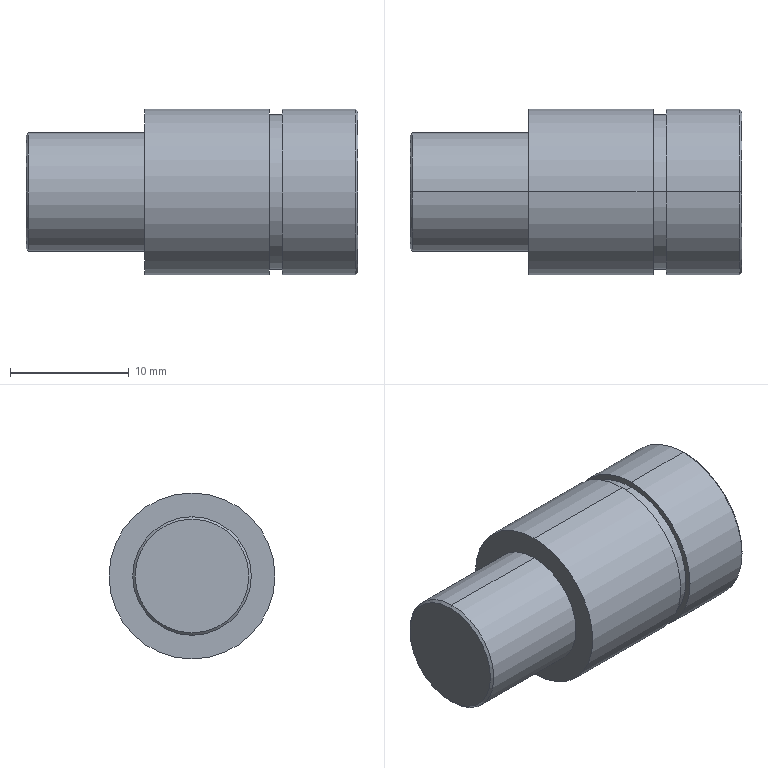Part | SolidWorks | features Chamfer 2, ICE 2, RevCut 1, Revolution 1 | 1 solid | 17 faces | box 28 x 14 x 14 mm | volume 3531 mm3 | cylinder 8 | plane 5 | cone 4 | commonest cylinder face diameters 14 x4 10 x2 13 x2
STEP:
#1=CARTESIAN_POINT('',(27.8,0.,7.));
#2=VERTEX_POINT('',#1);
#3=CARTESIAN_POINT('',(27.8,0.,-7.));
#4=VERTEX_POINT('',#3);
#5=CARTESIAN_POINT('',(27.8,0.,0.));
#6=DIRECTION('',(-1.,0.,0.));
#7=DIRECTION('',(0.,0.,1.));
#8=AXIS2_PLACEMENT_3D('',#5,#6,#7);
#9=CIRCLE('',#8,7.);
#10=EDGE_CURVE('',#2,#4,#9,.T.);
#11=ORIENTED_EDGE('',*,*,#10,.T.);
#12=CARTESIAN_POINT('',(21.6,0.,-7.));
#13=VERTEX_POINT('',#12);
#14=CARTESIAN_POINT('',(0.,0.,-7.));
#15=DIRECTION('',(-1.,0.,0.));
#16=VECTOR('',#15,1000.);
#17=LINE('',#14,#16);
#18=EDGE_CURVE('',#4,#13,#17,.T.);
#19=ORIENTED_EDGE('',*,*,#18,.T.);
#20=CARTESIAN_POINT('',(21.6,0.,7.));
#21=VERTEX_POINT('',#20);
#22=CARTESIAN_POINT('',(21.6,0.,0.));
#23=DIRECTION('',(-1.,0.,0.));
#24=DIRECTION('',(0.,0.,1.));
#25=AXIS2_PLACEMENT_3D('',#22,#23,#24);
#26=CIRCLE('',#25,7.);
#27=EDGE_CURVE('',#21,#13,#26,.T.);
#28=ORIENTED_EDGE('',*,*,#27,.F.);
#29=CARTESIAN_POINT('',(0.,0.,7.));
#30=DIRECTION('',(-1.,0.,0.));
#31=VECTOR('',#30,1000.);
#32=LINE('',#29,#31);
#33=EDGE_CURVE('',#2,#21,#32,.T.);
#34=ORIENTED_EDGE('',*,*,#33,.F.);
#35=EDGE_LOOP('',(#11,#19,#28,#34));
#36=FACE_OUTER_BOUND('',#35,.T.);
#37=CARTESIAN_POINT('',(0.,0.,0.));
#38=DIRECTION('',(-1.,0.,0.));
#39=DIRECTION('',(0.,0.,1.));
#40=AXIS2_PLACEMENT_3D('',#37,#38,#39);
#41=CYLINDRICAL_SURFACE('',#40,7.);
#42=ADVANCED_FACE('',(#36),#41,.T.);
#43=CARTESIAN_POINT('',(28.,0.,-6.8));
#44=VERTEX_POINT('',#43);
#45=CARTESIAN_POINT('',(28.,0.,6.8));
#46=VERTEX_POINT('',#45);
#47=CARTESIAN_POINT('',(28.,0.,0.));
#48=DIRECTION('',(1.,0.,0.));
#49=DIRECTION('',(0.,0.,1.));
#50=AXIS2_PLACEMENT_3D('',#47,#48,#49);
#51=CIRCLE('',#50,6.8);
#52=EDGE_CURVE('',#44,#46,#51,.T.);
#53=ORIENTED_EDGE('',*,*,#52,.F.);
#54=CARTESIAN_POINT('',(27.8,0.,-7.));
#55=DIRECTION('',(-0.7071,0.,-0.7071));
#56=VECTOR('',#55,1000.);
#57=LINE('',#54,#56);
#58=EDGE_CURVE('',#44,#4,#57,.T.);
#59=ORIENTED_EDGE('',*,*,#58,.T.);
#60=ORIENTED_EDGE('',*,*,#10,.F.);
#61=CARTESIAN_POINT('',(27.8,0.,7.));
#62=DIRECTION('',(-0.7071,0.,0.7071));
#63=VECTOR('',#62,1000.);
#64=LINE('',#61,#63);
#65=EDGE_CURVE('',#46,#2,#64,.T.);
#66=ORIENTED_EDGE('',*,*,#65,.F.);
#67=EDGE_LOOP('',(#53,#59,#60,#66));
#68=FACE_OUTER_BOUND('',#67,.T.);
#69=CARTESIAN_POINT('',(27.8,0.,0.));
#70=DIRECTION('',(-1.,0.,0.));
#71=DIRECTION('',(0.,0.,1.));
#72=AXIS2_PLACEMENT_3D('',#69,#70,#71);
#73=CONICAL_SURFACE('',#72,7.,0.7854);
#74=ADVANCED_FACE('',(#68),#73,.T.);
#75=CARTESIAN_POINT('',(21.6,0.,6.5));
#76=VERTEX_POINT('',#75);
#77=CARTESIAN_POINT('',(21.6,0.,-6.5));
#78=VERTEX_POINT('',#77);
#79=CARTESIAN_POINT('',(21.6,0.,0.));
#80=DIRECTION('',(-1.,0.,0.));
#81=DIRECTION('',(0.,0.,1.));
#82=AXIS2_PLACEMENT_3D('',#79,#80,#81);
#83=CIRCLE('',#82,6.5);
#84=EDGE_CURVE('',#76,#78,#83,.T.);
#85=ORIENTED_EDGE('',*,*,#84,.T.);
#86=CARTESIAN_POINT('',(20.5,0.,-6.5));
#87=VERTEX_POINT('',#86);
#88=CARTESIAN_POINT('',(0.,0.,-6.5));
#89=DIRECTION('',(-1.,0.,0.));
#90=VECTOR('',#89,1000.);
#91=LINE('',#88,#90);
#92=EDGE_CURVE('',#78,#87,#91,.T.);
#93=ORIENTED_EDGE('',*,*,#92,.T.);
#94=CARTESIAN_POINT('',(20.5,0.,6.5));
#95=VERTEX_POINT('',#94);
#96=CARTESIAN_POINT('',(20.5,0.,0.));
#97=DIRECTION('',(-1.,0.,0.));
#98=DIRECTION('',(0.,0.,1.));
#99=AXIS2_PLACEMENT_3D('',#96,#97,#98);
#100=CIRCLE('',#99,6.5);
#101=EDGE_CURVE('',#95,#87,#100,.T.);
#102=ORIENTED_EDGE('',*,*,#101,.F.);
#103=CARTESIAN_POINT('',(0.,0.,6.5));
#104=DIRECTION('',(-1.,0.,0.));
#105=VECTOR('',#104,1000.);
#106=LINE('',#103,#105);
#107=EDGE_CURVE('',#76,#95,#106,.T.);
#108=ORIENTED_EDGE('',*,*,#107,.F.);
#109=EDGE_LOOP('',(#85,#93,#102,#108));
#110=FACE_OUTER_BOUND('',#109,.T.);
#111=CARTESIAN_POINT('',(0.,0.,0.));
#112=DIRECTION('',(-1.,0.,0.));
#113=DIRECTION('',(0.,0.,1.));
#114=AXIS2_PLACEMENT_3D('',#111,#112,#113);
#115=CYLINDRICAL_SURFACE('',#114,6.5);
#116=ADVANCED_FACE('',(#110),#115,.T.);
#117=CARTESIAN_POINT('',(0.,0.,4.8));
#118=VERTEX_POINT('',#117);
#119=CARTESIAN_POINT('',(0.,0.,-4.8));
#120=VERTEX_POINT('',#119);
#121=CARTESIAN_POINT('',(0.,0.,0.));
#122=DIRECTION('',(-1.,0.,0.));
#123=DIRECTION('',(0.,0.,-1.));
#124=AXIS2_PLACEMENT_3D('',#121,#122,#123);
#125=CIRCLE('',#124,4.8);
#126=EDGE_CURVE('',#118,#120,#125,.T.);
#127=ORIENTED_EDGE('',*,*,#126,.F.);
#128=CARTESIAN_POINT('',(0.2,0.,5.));
#129=VERTEX_POINT('',#128);
#130=CARTESIAN_POINT('',(0.,0.,4.8));
#131=DIRECTION('',(0.7071,0.,0.7071));
#132=VECTOR('',#131,1000.);
#133=LINE('',#130,#132);
#134=EDGE_CURVE('',#118,#129,#133,.T.);
#135=ORIENTED_EDGE('',*,*,#134,.T.);
#136=CARTESIAN_POINT('',(0.2,0.,-5.));
#137=VERTEX_POINT('',#136);
#138=CARTESIAN_POINT('',(0.2,0.,0.));
#139=DIRECTION('',(1.,0.,0.));
#140=DIRECTION('',(0.,0.,-1.));
#141=AXIS2_PLACEMENT_3D('',#138,#139,#140);
#142=CIRCLE('',#141,5.);
#143=EDGE_CURVE('',#137,#129,#142,.T.);
#144=ORIENTED_EDGE('',*,*,#143,.F.);
#145=CARTESIAN_POINT('',(0.,0.,-4.8));
#146=DIRECTION('',(0.7071,0.,-0.7071));
#147=VECTOR('',#146,1000.);
#148=LINE('',#145,#147);
#149=EDGE_CURVE('',#120,#137,#148,.T.);
#150=ORIENTED_EDGE('',*,*,#149,.F.);
#151=EDGE_LOOP('',(#127,#135,#144,#150));
#152=FACE_OUTER_BOUND('',#151,.T.);
#153=CARTESIAN_POINT('',(0.,0.,0.));
#154=DIRECTION('',(1.,0.,0.));
#155=DIRECTION('',(0.,0.,-1.));
#156=AXIS2_PLACEMENT_3D('',#153,#154,#155);
#157=CONICAL_SURFACE('',#156,4.8,0.7854);
#158=ADVANCED_FACE('',(#152),#157,.T.);
#159=CARTESIAN_POINT('',(10.,0.,5.));
#160=VERTEX_POINT('',#159);
#161=CARTESIAN_POINT('',(10.,0.,-5.));
#162=VERTEX_POINT('',#161);
#163=CARTESIAN_POINT('',(10.,0.,0.));
#164=DIRECTION('',(-1.,0.,0.));
#165=DIRECTION('',(0.,0.,1.));
#166=AXIS2_PLACEMENT_3D('',#163,#164,#165);
#167=CIRCLE('',#166,5.);
#168=EDGE_CURVE('',#160,#162,#167,.T.);
#169=ORIENTED_EDGE('',*,*,#168,.T.);
#170=CARTESIAN_POINT('',(0.,0.,-5.));
#171=DIRECTION('',(-1.,0.,0.));
#172=VECTOR('',#171,1000.);
#173=LINE('',#170,#172);
#174=EDGE_CURVE('',#162,#137,#173,.T.);
#175=ORIENTED_EDGE('',*,*,#174,.T.);
#176=ORIENTED_EDGE('',*,*,#143,.T.);
#177=CARTESIAN_POINT('',(0.,0.,5.));
#178=DIRECTION('',(-1.,0.,0.));
#179=VECTOR('',#178,1000.);
#180=LINE('',#177,#179);
#181=EDGE_CURVE('',#160,#129,#180,.T.);
#182=ORIENTED_EDGE('',*,*,#181,.F.);
#183=EDGE_LOOP('',(#169,#175,#176,#182));
#184=FACE_OUTER_BOUND('',#183,.T.);
#185=CARTESIAN_POINT('',(0.,0.,0.));
#186=DIRECTION('',(-1.,0.,0.));
#187=DIRECTION('',(0.,0.,1.));
#188=AXIS2_PLACEMENT_3D('',#185,#186,#187);
#189=CYLINDRICAL_SURFACE('',#188,5.);
#190=ADVANCED_FACE('',(#184),#189,.T.);
#191=CARTESIAN_POINT('',(20.5,0.,-7.));
#192=VERTEX_POINT('',#191);
#193=CARTESIAN_POINT('',(20.5,0.,7.));
#194=VERTEX_POINT('',#193);
#195=CARTESIAN_POINT('',(20.5,0.,0.));
#196=DIRECTION('',(1.,0.,0.));
#197=DIRECTION('',(0.,0.,-1.));
#198=AXIS2_PLACEMENT_3D('',#195,#196,#197);
#199=CIRCLE('',#198,7.);
#200=EDGE_CURVE('',#192,#194,#199,.T.);
#201=ORIENTED_EDGE('',*,*,#200,.F.);
#202=CARTESIAN_POINT('',(10.,0.,-7.));
#203=VERTEX_POINT('',#202);
#204=CARTESIAN_POINT('',(0.,0.,-7.));
#205=DIRECTION('',(-1.,0.,0.));
#206=VECTOR('',#205,1000.);
#207=LINE('',#204,#206);
#208=EDGE_CURVE('',#192,#203,#207,.T.);
#209=ORIENTED_EDGE('',*,*,#208,.T.);
#210=CARTESIAN_POINT('',(10.,0.,7.));
#211=VERTEX_POINT('',#210);
#212=CARTESIAN_POINT('',(10.,0.,0.));
#213=DIRECTION('',(-1.,0.,0.));
#214=DIRECTION('',(0.,0.,1.));
#215=AXIS2_PLACEMENT_3D('',#212,#213,#214);
#216=CIRCLE('',#215,7.);
#217=EDGE_CURVE('',#211,#203,#216,.T.);
#218=ORIENTED_EDGE('',*,*,#217,.F.);
#219=CARTESIAN_POINT('',(0.,0.,7.));
#220=DIRECTION('',(-1.,0.,0.));
#221=VECTOR('',#220,1000.);
#222=LINE('',#219,#221);
#223=EDGE_CURVE('',#194,#211,#222,.T.);
#224=ORIENTED_EDGE('',*,*,#223,.F.);
#225=EDGE_LOOP('',(#201,#209,#218,#224));
#226=FACE_OUTER_BOUND('',#225,.T.);
#227=CARTESIAN_POINT('',(0.,0.,0.));
#228=DIRECTION('',(-1.,0.,0.));
#229=DIRECTION('',(0.,0.,1.));
#230=AXIS2_PLACEMENT_3D('',#227,#228,#229);
#231=CYLINDRICAL_SURFACE('',#230,7.);
#232=ADVANCED_FACE('',(#226),#231,.T.);
#233=ORIENTED_EDGE('',*,*,#208,.F.);
#234=CARTESIAN_POINT('',(20.5,0.,0.));
#235=DIRECTION('',(1.,0.,0.));
#236=DIRECTION('',(0.,0.,-1.));
#237=AXIS2_PLACEMENT_3D('',#234,#235,#236);
#238=CIRCLE('',#237,7.);
#239=EDGE_CURVE('',#194,#192,#238,.T.);
#240=ORIENTED_EDGE('',*,*,#239,.F.);
#241=ORIENTED_EDGE('',*,*,#223,.T.);
#242=CARTESIAN_POINT('',(10.,0.,0.));
#243=DIRECTION('',(-1.,0.,0.));
#244=DIRECTION('',(0.,0.,1.));
#245=AXIS2_PLACEMENT_3D('',#242,#243,#244);
#246=CIRCLE('',#245,7.);
#247=EDGE_CURVE('',#203,#211,#246,.T.);
#248=ORIENTED_EDGE('',*,*,#247,.F.);
#249=EDGE_LOOP('',(#233,#240,#241,#248));
#250=FACE_OUTER_BOUND('',#249,.T.);
#251=CARTESIAN_POINT('',(0.,0.,0.));
#252=DIRECTION('',(-1.,0.,0.));
#253=DIRECTION('',(0.,0.,1.));
#254=AXIS2_PLACEMENT_3D('',#251,#252,#253);
#255=CYLINDRICAL_SURFACE('',#254,7.);
#256=ADVANCED_FACE('',(#250),#255,.T.);
#257=CARTESIAN_POINT('',(0.,0.,0.));
#258=DIRECTION('',(-1.,0.,0.));
#259=DIRECTION('',(0.,0.,-1.));
#260=AXIS2_PLACEMENT_3D('',#257,#258,#259);
#261=CIRCLE('',#260,4.8);
#262=EDGE_CURVE('',#120,#118,#261,.T.);
#263=ORIENTED_EDGE('',*,*,#262,.T.);
#264=ORIENTED_EDGE('',*,*,#126,.T.);
#265=EDGE_LOOP('',(#263,#264));
#266=FACE_OUTER_BOUND('',#265,.T.);
#267=CARTESIAN_POINT('',(0.,0.,0.));
#268=DIRECTION('',(1.,0.,0.));
#269=DIRECTION('',(0.,0.,-1.));
#270=AXIS2_PLACEMENT_3D('',#267,#268,#269);
#271=PLANE('',#270);
#272=ADVANCED_FACE('',(#266),#271,.F.);
#273=ORIENTED_EDGE('',*,*,#174,.F.);
#274=CARTESIAN_POINT('',(10.,0.,0.));
#275=DIRECTION('',(-1.,0.,0.));
#276=DIRECTION('',(0.,0.,1.));
#277=AXIS2_PLACEMENT_3D('',#274,#275,#276);
#278=CIRCLE('',#277,5.);
#279=EDGE_CURVE('',#162,#160,#278,.T.);
#280=ORIENTED_EDGE('',*,*,#279,.T.);
#281=ORIENTED_EDGE('',*,*,#181,.T.);
#282=CARTESIAN_POINT('',(0.2,0.,0.));
#283=DIRECTION('',(1.,0.,0.));
#284=DIRECTION('',(0.,0.,-1.));
#285=AXIS2_PLACEMENT_3D('',#282,#283,#284);
#286=CIRCLE('',#285,5.);
#287=EDGE_CURVE('',#129,#137,#286,.T.);
#288=ORIENTED_EDGE('',*,*,#287,.T.);
#289=EDGE_LOOP('',(#273,#280,#281,#288));
#290=FACE_OUTER_BOUND('',#289,.T.);
#291=CARTESIAN_POINT('',(0.,0.,0.));
#292=DIRECTION('',(-1.,0.,0.));
#293=DIRECTION('',(0.,0.,1.));
#294=AXIS2_PLACEMENT_3D('',#291,#292,#293);
#295=CYLINDRICAL_SURFACE('',#294,5.);
#296=ADVANCED_FACE('',(#290),#295,.T.);
#297=ORIENTED_EDGE('',*,*,#168,.F.);
#298=ORIENTED_EDGE('',*,*,#279,.F.);
#299=EDGE_LOOP('',(#297,#298));
#300=FACE_BOUND('',#299,.T.);
#301=ORIENTED_EDGE('',*,*,#217,.T.);
#302=ORIENTED_EDGE('',*,*,#247,.T.);
#303=EDGE_LOOP('',(#301,#302));
#304=FACE_OUTER_BOUND('',#303,.T.);
#305=CARTESIAN_POINT('',(10.,5.,0.));
#306=DIRECTION('',(1.,0.,0.));
#307=DIRECTION('',(0.,0.,-1.));
#308=AXIS2_PLACEMENT_3D('',#305,#306,#307);
#309=PLANE('',#308);
#310=ADVANCED_FACE('',(#300,#304),#309,.F.);
#311=ORIENTED_EDGE('',*,*,#134,.F.);
#312=ORIENTED_EDGE('',*,*,#262,.F.);
#313=ORIENTED_EDGE('',*,*,#149,.T.);
#314=ORIENTED_EDGE('',*,*,#287,.F.);
#315=EDGE_LOOP('',(#311,#312,#313,#314));
#316=FACE_OUTER_BOUND('',#315,.T.);
#317=CARTESIAN_POINT('',(0.,0.,0.));
#318=DIRECTION('',(1.,0.,0.));
#319=DIRECTION('',(0.,0.,-1.));
#320=AXIS2_PLACEMENT_3D('',#317,#318,#319);
#321=CONICAL_SURFACE('',#320,4.8,0.7854);
#322=ADVANCED_FACE('',(#316),#321,.T.);
#323=ORIENTED_EDGE('',*,*,#101,.T.);
#324=CARTESIAN_POINT('',(20.5,0.,0.));
#325=DIRECTION('',(-1.,0.,0.));
#326=DIRECTION('',(0.,0.,1.));
#327=AXIS2_PLACEMENT_3D('',#324,#325,#326);
#328=CIRCLE('',#327,6.5);
#329=EDGE_CURVE('',#87,#95,#328,.T.);
#330=ORIENTED_EDGE('',*,*,#329,.T.);
#331=EDGE_LOOP('',(#323,#330));
#332=FACE_BOUND('',#331,.T.);
#333=ORIENTED_EDGE('',*,*,#239,.T.);
#334=ORIENTED_EDGE('',*,*,#200,.T.);
#335=EDGE_LOOP('',(#333,#334));
#336=FACE_OUTER_BOUND('',#335,.T.);
#337=CARTESIAN_POINT('',(20.5,0.,-8.894));
#338=DIRECTION('',(1.,0.,0.));
#339=DIRECTION('',(0.,0.,-1.));
#340=AXIS2_PLACEMENT_3D('',#337,#338,#339);
#341=PLANE('',#340);
#342=ADVANCED_FACE('',(#332,#336),#341,.T.);
#343=ORIENTED_EDGE('',*,*,#84,.F.);
#344=CARTESIAN_POINT('',(21.6,0.,0.));
#345=DIRECTION('',(-1.,0.,0.));
#346=DIRECTION('',(0.,0.,1.));
#347=AXIS2_PLACEMENT_3D('',#344,#345,#346);
#348=CIRCLE('',#347,6.5);
#349=EDGE_CURVE('',#78,#76,#348,.T.);
#350=ORIENTED_EDGE('',*,*,#349,.F.);
#351=EDGE_LOOP('',(#343,#350));
#352=FACE_BOUND('',#351,.T.);
#353=ORIENTED_EDGE('',*,*,#27,.T.);
#354=CARTESIAN_POINT('',(21.6,0.,0.));
#355=DIRECTION('',(-1.,0.,0.));
#356=DIRECTION('',(0.,0.,1.));
#357=AXIS2_PLACEMENT_3D('',#354,#355,#356);
#358=CIRCLE('',#357,7.);
#359=EDGE_CURVE('',#13,#21,#358,.T.);
#360=ORIENTED_EDGE('',*,*,#359,.T.);
#361=EDGE_LOOP('',(#353,#360));
#362=FACE_OUTER_BOUND('',#361,.T.);
#363=CARTESIAN_POINT('',(21.6,0.,-8.894));
#364=DIRECTION('',(-1.,0.,0.));
#365=DIRECTION('',(0.,0.,1.));
#366=AXIS2_PLACEMENT_3D('',#363,#364,#365);
#367=PLANE('',#366);
#368=ADVANCED_FACE('',(#352,#362),#367,.T.);
#369=ORIENTED_EDGE('',*,*,#92,.F.);
#370=ORIENTED_EDGE('',*,*,#349,.T.);
#371=ORIENTED_EDGE('',*,*,#107,.T.);
#372=ORIENTED_EDGE('',*,*,#329,.F.);
#373=EDGE_LOOP('',(#369,#370,#371,#372));
#374=FACE_OUTER_BOUND('',#373,.T.);
#375=CARTESIAN_POINT('',(0.,0.,0.));
#376=DIRECTION('',(-1.,0.,0.));
#377=DIRECTION('',(0.,0.,1.));
#378=AXIS2_PLACEMENT_3D('',#375,#376,#377);
#379=CYLINDRICAL_SURFACE('',#378,6.5);
#380=ADVANCED_FACE('',(#374),#379,.T.);
#381=CARTESIAN_POINT('',(28.,0.,0.));
#382=DIRECTION('',(1.,0.,0.));
#383=DIRECTION('',(0.,0.,1.));
#384=AXIS2_PLACEMENT_3D('',#381,#382,#383);
#385=CIRCLE('',#384,6.8);
#386=EDGE_CURVE('',#46,#44,#385,.T.);
#387=ORIENTED_EDGE('',*,*,#386,.T.);
#388=ORIENTED_EDGE('',*,*,#52,.T.);
#389=EDGE_LOOP('',(#387,#388));
#390=FACE_OUTER_BOUND('',#389,.T.);
#391=CARTESIAN_POINT('',(28.,7.,0.));
#392=DIRECTION('',(-1.,0.,0.));
#393=DIRECTION('',(0.,0.,1.));
#394=AXIS2_PLACEMENT_3D('',#391,#392,#393);
#395=PLANE('',#394);
#396=ADVANCED_FACE('',(#390),#395,.F.);
#397=ORIENTED_EDGE('',*,*,#58,.F.);
#398=ORIENTED_EDGE('',*,*,#386,.F.);
#399=ORIENTED_EDGE('',*,*,#65,.T.);
#400=CARTESIAN_POINT('',(27.8,0.,0.));
#401=DIRECTION('',(-1.,0.,0.));
#402=DIRECTION('',(0.,0.,1.));
#403=AXIS2_PLACEMENT_3D('',#400,#401,#402);
#404=CIRCLE('',#403,7.);
#405=EDGE_CURVE('',#4,#2,#404,.T.);
#406=ORIENTED_EDGE('',*,*,#405,.F.);
#407=EDGE_LOOP('',(#397,#398,#399,#406));
#408=FACE_OUTER_BOUND('',#407,.T.);
#409=CARTESIAN_POINT('',(27.8,0.,0.));
#410=DIRECTION('',(-1.,0.,0.));
#411=DIRECTION('',(0.,0.,1.));
#412=AXIS2_PLACEMENT_3D('',#409,#410,#411);
#413=CONICAL_SURFACE('',#412,7.,0.7854);
#414=ADVANCED_FACE('',(#408),#413,.T.);
#415=ORIENTED_EDGE('',*,*,#18,.F.);
#416=ORIENTED_EDGE('',*,*,#405,.T.);
#417=ORIENTED_EDGE('',*,*,#33,.T.);
#418=ORIENTED_EDGE('',*,*,#359,.F.);
#419=EDGE_LOOP('',(#415,#416,#417,#418));
#420=FACE_OUTER_BOUND('',#419,.T.);
#421=CARTESIAN_POINT('',(0.,0.,0.));
#422=DIRECTION('',(-1.,0.,0.));
#423=DIRECTION('',(0.,0.,1.));
#424=AXIS2_PLACEMENT_3D('',#421,#422,#423);
#425=CYLINDRICAL_SURFACE('',#424,7.);
#426=ADVANCED_FACE('',(#420),#425,.T.);
#427=CLOSED_SHELL('',(#42,#74,#116,#158,#190,#232,#256,#272,#296,#310,#322,#342,#368,#380,#396,#414,#426));
#428=MANIFOLD_SOLID_BREP('',#427);
#429=CARTESIAN_POINT('',(0.,0.,0.));
#430=DIRECTION('',(0.,0.,1.));
#431=DIRECTION('',(1.,0.,0.));
#432=AXIS2_PLACEMENT_3D('',#429,#430,#431);
#433=(LENGTH_UNIT()NAMED_UNIT(*)SI_UNIT(.MILLI.,.METRE.));
#434=UNCERTAINTY_MEASURE_WITH_UNIT(LENGTH_MEASURE(0.00001),#433,'','');
#435=(NAMED_UNIT(*)PLANE_ANGLE_UNIT()SI_UNIT($,.RADIAN.));
#436=(NAMED_UNIT(*)SI_UNIT($,.STERADIAN.)SOLID_ANGLE_UNIT());
#437=(GEOMETRIC_REPRESENTATION_CONTEXT(3)GLOBAL_UNCERTAINTY_ASSIGNED_CONTEXT((#434))GLOBAL_UNIT_ASSIGNED_CONTEXT((#433,#435,#436))REPRESENTATION_CONTEXT('',''));
#438=ADVANCED_BREP_SHAPE_REPRESENTATION('',(#428,#432),#437);